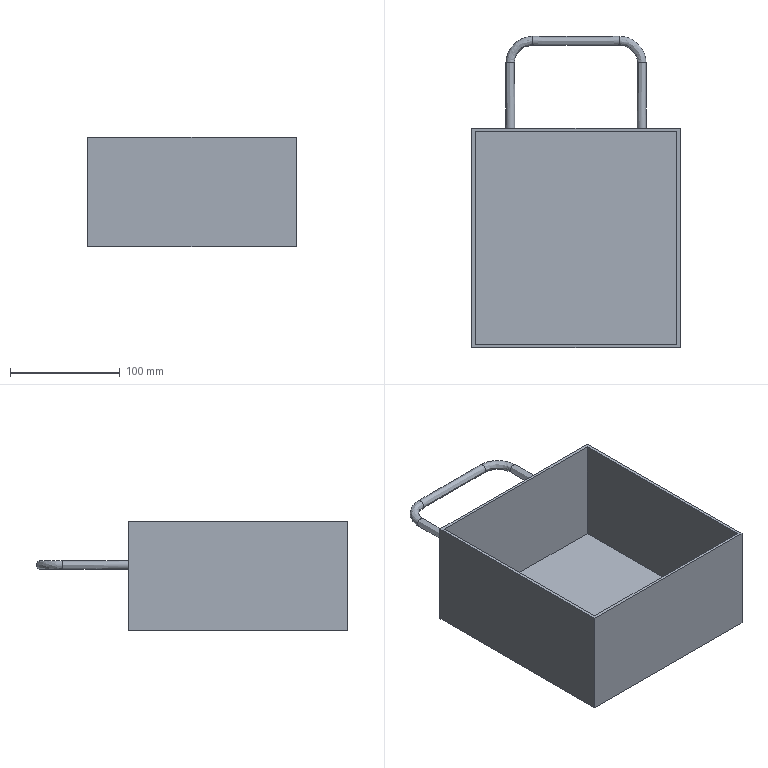Part | NX | features solid 2 | 1 solid | 16 faces | box 190 x 284 x 100 mm | volume 350706 mm3 | plane 11 | spline 5